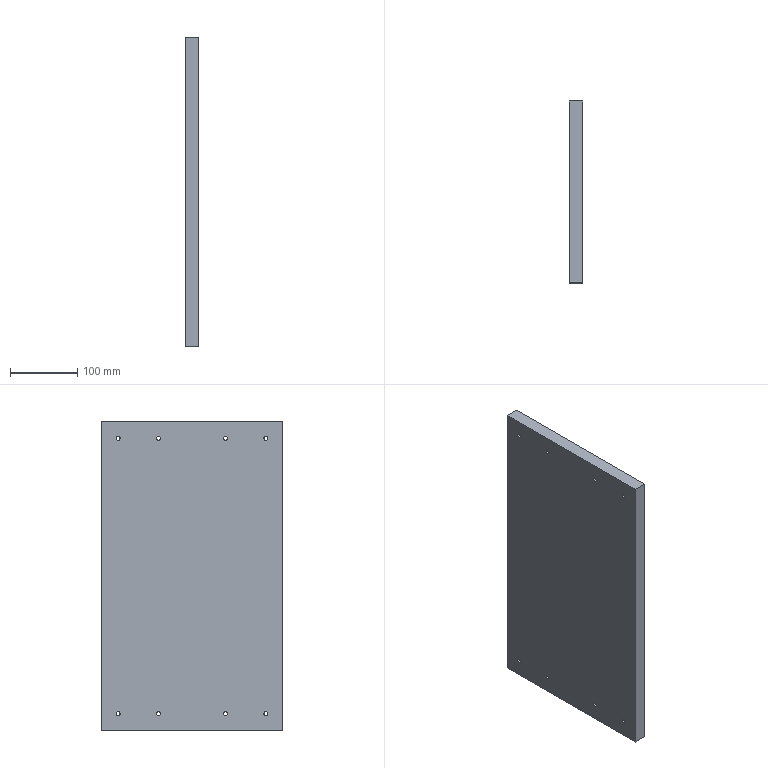Part | STEP file | Cut-Extrude 1 | 1 solid | 22 faces | box 20 x 270 x 460 mm | volume 2479476 mm3 | cylinder 16 | plane 6 | commonest cylinder face diameters 6 x16
STEP:
#1=CARTESIAN_POINT('',(-1338.738,1924.264,3010.5));
#2=VERTEX_POINT('',#1);
#3=CARTESIAN_POINT('',(-1338.738,1924.264,3016.5));
#4=VERTEX_POINT('',#3);
#5=CARTESIAN_POINT('',(-1338.738,1924.264,3013.5));
#6=DIRECTION('',(-1.,0.,0.));
#7=DIRECTION('',(0.,0.,1.));
#8=AXIS2_PLACEMENT_3D('',#5,#6,#7);
#9=CIRCLE('',#8,3.);
#10=EDGE_CURVE('',#2,#4,#9,.T.);
#11=ORIENTED_EDGE('',*,*,#10,.F.);
#12=CARTESIAN_POINT('',(-1358.738,1924.264,3010.5));
#13=VERTEX_POINT('',#12);
#14=CARTESIAN_POINT('',(-1269.738,1924.264,3010.5));
#15=DIRECTION('',(-1.,0.,0.));
#16=VECTOR('',#15,1000.);
#17=LINE('',#14,#16);
#18=EDGE_CURVE('',#2,#13,#17,.T.);
#19=ORIENTED_EDGE('',*,*,#18,.T.);
#20=CARTESIAN_POINT('',(-1358.738,1924.264,3016.5));
#21=VERTEX_POINT('',#20);
#22=CARTESIAN_POINT('',(-1358.738,1924.264,3013.5));
#23=DIRECTION('',(-1.,0.,0.));
#24=DIRECTION('',(0.,0.,-1.));
#25=AXIS2_PLACEMENT_3D('',#22,#23,#24);
#26=CIRCLE('',#25,3.);
#27=EDGE_CURVE('',#13,#21,#26,.T.);
#28=ORIENTED_EDGE('',*,*,#27,.T.);
#29=CARTESIAN_POINT('',(-1269.738,1924.264,3016.5));
#30=DIRECTION('',(-1.,0.,0.));
#31=VECTOR('',#30,1000.);
#32=LINE('',#29,#31);
#33=EDGE_CURVE('',#4,#21,#32,.T.);
#34=ORIENTED_EDGE('',*,*,#33,.F.);
#35=EDGE_LOOP('',(#11,#19,#28,#34));
#36=FACE_OUTER_BOUND('',#35,.T.);
#37=CARTESIAN_POINT('',(-1269.738,1924.264,3013.5));
#38=DIRECTION('',(-1.,0.,0.));
#39=DIRECTION('',(0.,0.,-1.));
#40=AXIS2_PLACEMENT_3D('',#37,#38,#39);
#41=CYLINDRICAL_SURFACE('',#40,3.);
#42=ADVANCED_FACE('',(#36),#41,.F.);
#43=CARTESIAN_POINT('',(-1338.738,1864.264,3010.5));
#44=VERTEX_POINT('',#43);
#45=CARTESIAN_POINT('',(-1338.738,1864.264,3016.5));
#46=VERTEX_POINT('',#45);
#47=CARTESIAN_POINT('',(-1338.738,1864.264,3013.5));
#48=DIRECTION('',(-1.,0.,0.));
#49=DIRECTION('',(0.,0.,1.));
#50=AXIS2_PLACEMENT_3D('',#47,#48,#49);
#51=CIRCLE('',#50,3.);
#52=EDGE_CURVE('',#44,#46,#51,.T.);
#53=ORIENTED_EDGE('',*,*,#52,.F.);
#54=CARTESIAN_POINT('',(-1358.738,1864.264,3010.5));
#55=VERTEX_POINT('',#54);
#56=CARTESIAN_POINT('',(-1269.738,1864.264,3010.5));
#57=DIRECTION('',(-1.,0.,0.));
#58=VECTOR('',#57,1000.);
#59=LINE('',#56,#58);
#60=EDGE_CURVE('',#44,#55,#59,.T.);
#61=ORIENTED_EDGE('',*,*,#60,.T.);
#62=CARTESIAN_POINT('',(-1358.738,1864.264,3016.5));
#63=VERTEX_POINT('',#62);
#64=CARTESIAN_POINT('',(-1358.738,1864.264,3013.5));
#65=DIRECTION('',(-1.,0.,0.));
#66=DIRECTION('',(0.,0.,-1.));
#67=AXIS2_PLACEMENT_3D('',#64,#65,#66);
#68=CIRCLE('',#67,3.);
#69=EDGE_CURVE('',#55,#63,#68,.T.);
#70=ORIENTED_EDGE('',*,*,#69,.T.);
#71=CARTESIAN_POINT('',(-1269.738,1864.264,3016.5));
#72=DIRECTION('',(-1.,0.,0.));
#73=VECTOR('',#72,1000.);
#74=LINE('',#71,#73);
#75=EDGE_CURVE('',#46,#63,#74,.T.);
#76=ORIENTED_EDGE('',*,*,#75,.F.);
#77=EDGE_LOOP('',(#53,#61,#70,#76));
#78=FACE_OUTER_BOUND('',#77,.T.);
#79=CARTESIAN_POINT('',(-1269.738,1864.264,3013.5));
#80=DIRECTION('',(-1.,0.,0.));
#81=DIRECTION('',(0.,0.,-1.));
#82=AXIS2_PLACEMENT_3D('',#79,#80,#81);
#83=CYLINDRICAL_SURFACE('',#82,3.);
#84=ADVANCED_FACE('',(#78),#83,.F.);
#85=CARTESIAN_POINT('',(-1338.738,1764.264,3010.5));
#86=VERTEX_POINT('',#85);
#87=CARTESIAN_POINT('',(-1338.738,1764.264,3016.5));
#88=VERTEX_POINT('',#87);
#89=CARTESIAN_POINT('',(-1338.738,1764.264,3013.5));
#90=DIRECTION('',(-1.,0.,0.));
#91=DIRECTION('',(0.,0.,1.));
#92=AXIS2_PLACEMENT_3D('',#89,#90,#91);
#93=CIRCLE('',#92,3.);
#94=EDGE_CURVE('',#86,#88,#93,.T.);
#95=ORIENTED_EDGE('',*,*,#94,.F.);
#96=CARTESIAN_POINT('',(-1358.738,1764.264,3010.5));
#97=VERTEX_POINT('',#96);
#98=CARTESIAN_POINT('',(-1269.738,1764.264,3010.5));
#99=DIRECTION('',(-1.,0.,0.));
#100=VECTOR('',#99,1000.);
#101=LINE('',#98,#100);
#102=EDGE_CURVE('',#86,#97,#101,.T.);
#103=ORIENTED_EDGE('',*,*,#102,.T.);
#104=CARTESIAN_POINT('',(-1358.738,1764.264,3016.5));
#105=VERTEX_POINT('',#104);
#106=CARTESIAN_POINT('',(-1358.738,1764.264,3013.5));
#107=DIRECTION('',(-1.,0.,0.));
#108=DIRECTION('',(0.,0.,1.));
#109=AXIS2_PLACEMENT_3D('',#106,#107,#108);
#110=CIRCLE('',#109,3.);
#111=EDGE_CURVE('',#97,#105,#110,.T.);
#112=ORIENTED_EDGE('',*,*,#111,.T.);
#113=CARTESIAN_POINT('',(-1269.738,1764.264,3016.5));
#114=DIRECTION('',(-1.,0.,0.));
#115=VECTOR('',#114,1000.);
#116=LINE('',#113,#115);
#117=EDGE_CURVE('',#88,#105,#116,.T.);
#118=ORIENTED_EDGE('',*,*,#117,.F.);
#119=EDGE_LOOP('',(#95,#103,#112,#118));
#120=FACE_OUTER_BOUND('',#119,.T.);
#121=CARTESIAN_POINT('',(-1269.738,1764.264,3013.5));
#122=DIRECTION('',(-1.,0.,0.));
#123=DIRECTION('',(0.,0.,-1.));
#124=AXIS2_PLACEMENT_3D('',#121,#122,#123);
#125=CYLINDRICAL_SURFACE('',#124,3.);
#126=ADVANCED_FACE('',(#120),#125,.F.);
#127=CARTESIAN_POINT('',(-1338.738,1704.264,3010.5));
#128=VERTEX_POINT('',#127);
#129=CARTESIAN_POINT('',(-1338.738,1704.264,3016.5));
#130=VERTEX_POINT('',#129);
#131=CARTESIAN_POINT('',(-1338.738,1704.264,3013.5));
#132=DIRECTION('',(-1.,0.,0.));
#133=DIRECTION('',(0.,0.,1.));
#134=AXIS2_PLACEMENT_3D('',#131,#132,#133);
#135=CIRCLE('',#134,3.);
#136=EDGE_CURVE('',#128,#130,#135,.T.);
#137=ORIENTED_EDGE('',*,*,#136,.F.);
#138=CARTESIAN_POINT('',(-1358.738,1704.264,3010.5));
#139=VERTEX_POINT('',#138);
#140=CARTESIAN_POINT('',(-1269.738,1704.264,3010.5));
#141=DIRECTION('',(-1.,0.,0.));
#142=VECTOR('',#141,1000.);
#143=LINE('',#140,#142);
#144=EDGE_CURVE('',#128,#139,#143,.T.);
#145=ORIENTED_EDGE('',*,*,#144,.T.);
#146=CARTESIAN_POINT('',(-1358.738,1704.264,3016.5));
#147=VERTEX_POINT('',#146);
#148=CARTESIAN_POINT('',(-1358.738,1704.264,3013.5));
#149=DIRECTION('',(-1.,0.,0.));
#150=DIRECTION('',(0.,0.,1.));
#151=AXIS2_PLACEMENT_3D('',#148,#149,#150);
#152=CIRCLE('',#151,3.);
#153=EDGE_CURVE('',#139,#147,#152,.T.);
#154=ORIENTED_EDGE('',*,*,#153,.T.);
#155=CARTESIAN_POINT('',(-1269.738,1704.264,3016.5));
#156=DIRECTION('',(-1.,0.,0.));
#157=VECTOR('',#156,1000.);
#158=LINE('',#155,#157);
#159=EDGE_CURVE('',#130,#147,#158,.T.);
#160=ORIENTED_EDGE('',*,*,#159,.F.);
#161=EDGE_LOOP('',(#137,#145,#154,#160));
#162=FACE_OUTER_BOUND('',#161,.T.);
#163=CARTESIAN_POINT('',(-1269.738,1704.264,3013.5));
#164=DIRECTION('',(-1.,0.,0.));
#165=DIRECTION('',(0.,0.,-1.));
#166=AXIS2_PLACEMENT_3D('',#163,#164,#165);
#167=CYLINDRICAL_SURFACE('',#166,3.);
#168=ADVANCED_FACE('',(#162),#167,.F.);
#169=CARTESIAN_POINT('',(-1338.738,1704.264,2600.5));
#170=VERTEX_POINT('',#169);
#171=CARTESIAN_POINT('',(-1338.738,1704.264,2606.5));
#172=VERTEX_POINT('',#171);
#173=CARTESIAN_POINT('',(-1338.738,1704.264,2603.5));
#174=DIRECTION('',(-1.,0.,0.));
#175=DIRECTION('',(0.,0.,1.));
#176=AXIS2_PLACEMENT_3D('',#173,#174,#175);
#177=CIRCLE('',#176,3.);
#178=EDGE_CURVE('',#170,#172,#177,.T.);
#179=ORIENTED_EDGE('',*,*,#178,.F.);
#180=CARTESIAN_POINT('',(-1358.738,1704.264,2600.5));
#181=VERTEX_POINT('',#180);
#182=CARTESIAN_POINT('',(-1269.738,1704.264,2600.5));
#183=DIRECTION('',(-1.,0.,0.));
#184=VECTOR('',#183,1000.);
#185=LINE('',#182,#184);
#186=EDGE_CURVE('',#170,#181,#185,.T.);
#187=ORIENTED_EDGE('',*,*,#186,.T.);
#188=CARTESIAN_POINT('',(-1358.738,1704.264,2606.5));
#189=VERTEX_POINT('',#188);
#190=CARTESIAN_POINT('',(-1358.738,1704.264,2603.5));
#191=DIRECTION('',(-1.,0.,0.));
#192=DIRECTION('',(0.,0.,-1.));
#193=AXIS2_PLACEMENT_3D('',#190,#191,#192);
#194=CIRCLE('',#193,3.);
#195=EDGE_CURVE('',#181,#189,#194,.T.);
#196=ORIENTED_EDGE('',*,*,#195,.T.);
#197=CARTESIAN_POINT('',(-1269.738,1704.264,2606.5));
#198=DIRECTION('',(-1.,0.,0.));
#199=VECTOR('',#198,1000.);
#200=LINE('',#197,#199);
#201=EDGE_CURVE('',#172,#189,#200,.T.);
#202=ORIENTED_EDGE('',*,*,#201,.F.);
#203=EDGE_LOOP('',(#179,#187,#196,#202));
#204=FACE_OUTER_BOUND('',#203,.T.);
#205=CARTESIAN_POINT('',(-1269.738,1704.264,2603.5));
#206=DIRECTION('',(-1.,0.,0.));
#207=DIRECTION('',(0.,0.,-1.));
#208=AXIS2_PLACEMENT_3D('',#205,#206,#207);
#209=CYLINDRICAL_SURFACE('',#208,3.);
#210=ADVANCED_FACE('',(#204),#209,.F.);
#211=CARTESIAN_POINT('',(-1338.738,1764.264,2600.5));
#212=VERTEX_POINT('',#211);
#213=CARTESIAN_POINT('',(-1338.738,1764.264,2606.5));
#214=VERTEX_POINT('',#213);
#215=CARTESIAN_POINT('',(-1338.738,1764.264,2603.5));
#216=DIRECTION('',(-1.,0.,0.));
#217=DIRECTION('',(0.,0.,1.));
#218=AXIS2_PLACEMENT_3D('',#215,#216,#217);
#219=CIRCLE('',#218,3.);
#220=EDGE_CURVE('',#212,#214,#219,.T.);
#221=ORIENTED_EDGE('',*,*,#220,.F.);
#222=CARTESIAN_POINT('',(-1358.738,1764.264,2600.5));
#223=VERTEX_POINT('',#222);
#224=CARTESIAN_POINT('',(-1269.738,1764.264,2600.5));
#225=DIRECTION('',(-1.,0.,0.));
#226=VECTOR('',#225,1000.);
#227=LINE('',#224,#226);
#228=EDGE_CURVE('',#212,#223,#227,.T.);
#229=ORIENTED_EDGE('',*,*,#228,.T.);
#230=CARTESIAN_POINT('',(-1358.738,1764.264,2606.5));
#231=VERTEX_POINT('',#230);
#232=CARTESIAN_POINT('',(-1358.738,1764.264,2603.5));
#233=DIRECTION('',(-1.,0.,0.));
#234=DIRECTION('',(0.,0.,-1.));
#235=AXIS2_PLACEMENT_3D('',#232,#233,#234);
#236=CIRCLE('',#235,3.);
#237=EDGE_CURVE('',#223,#231,#236,.T.);
#238=ORIENTED_EDGE('',*,*,#237,.T.);
#239=CARTESIAN_POINT('',(-1269.738,1764.264,2606.5));
#240=DIRECTION('',(-1.,0.,0.));
#241=VECTOR('',#240,1000.);
#242=LINE('',#239,#241);
#243=EDGE_CURVE('',#214,#231,#242,.T.);
#244=ORIENTED_EDGE('',*,*,#243,.F.);
#245=EDGE_LOOP('',(#221,#229,#238,#244));
#246=FACE_OUTER_BOUND('',#245,.T.);
#247=CARTESIAN_POINT('',(-1269.738,1764.264,2603.5));
#248=DIRECTION('',(-1.,0.,0.));
#249=DIRECTION('',(0.,0.,-1.));
#250=AXIS2_PLACEMENT_3D('',#247,#248,#249);
#251=CYLINDRICAL_SURFACE('',#250,3.);
#252=ADVANCED_FACE('',(#246),#251,.F.);
#253=CARTESIAN_POINT('',(-1338.738,1864.264,2600.5));
#254=VERTEX_POINT('',#253);
#255=CARTESIAN_POINT('',(-1338.738,1864.264,2606.5));
#256=VERTEX_POINT('',#255);
#257=CARTESIAN_POINT('',(-1338.738,1864.264,2603.5));
#258=DIRECTION('',(-1.,0.,0.));
#259=DIRECTION('',(0.,0.,1.));
#260=AXIS2_PLACEMENT_3D('',#257,#258,#259);
#261=CIRCLE('',#260,3.);
#262=EDGE_CURVE('',#254,#256,#261,.T.);
#263=ORIENTED_EDGE('',*,*,#262,.F.);
#264=CARTESIAN_POINT('',(-1358.738,1864.264,2600.5));
#265=VERTEX_POINT('',#264);
#266=CARTESIAN_POINT('',(-1269.738,1864.264,2600.5));
#267=DIRECTION('',(-1.,0.,0.));
#268=VECTOR('',#267,1000.);
#269=LINE('',#266,#268);
#270=EDGE_CURVE('',#254,#265,#269,.T.);
#271=ORIENTED_EDGE('',*,*,#270,.T.);
#272=CARTESIAN_POINT('',(-1358.738,1864.264,2606.5));
#273=VERTEX_POINT('',#272);
#274=CARTESIAN_POINT('',(-1358.738,1864.264,2603.5));
#275=DIRECTION('',(-1.,0.,0.));
#276=DIRECTION('',(0.,0.,1.));
#277=AXIS2_PLACEMENT_3D('',#274,#275,#276);
#278=CIRCLE('',#277,3.);
#279=EDGE_CURVE('',#265,#273,#278,.T.);
#280=ORIENTED_EDGE('',*,*,#279,.T.);
#281=CARTESIAN_POINT('',(-1269.738,1864.264,2606.5));
#282=DIRECTION('',(-1.,0.,0.));
#283=VECTOR('',#282,1000.);
#284=LINE('',#281,#283);
#285=EDGE_CURVE('',#256,#273,#284,.T.);
#286=ORIENTED_EDGE('',*,*,#285,.F.);
#287=EDGE_LOOP('',(#263,#271,#280,#286));
#288=FACE_OUTER_BOUND('',#287,.T.);
#289=CARTESIAN_POINT('',(-1269.738,1864.264,2603.5));
#290=DIRECTION('',(-1.,0.,0.));
#291=DIRECTION('',(0.,0.,-1.));
#292=AXIS2_PLACEMENT_3D('',#289,#290,#291);
#293=CYLINDRICAL_SURFACE('',#292,3.);
#294=ADVANCED_FACE('',(#288),#293,.F.);
#295=CARTESIAN_POINT('',(-1338.738,1924.264,2600.5));
#296=VERTEX_POINT('',#295);
#297=CARTESIAN_POINT('',(-1338.738,1924.264,2606.5));
#298=VERTEX_POINT('',#297);
#299=CARTESIAN_POINT('',(-1338.738,1924.264,2603.5));
#300=DIRECTION('',(-1.,0.,0.));
#301=DIRECTION('',(0.,0.,1.));
#302=AXIS2_PLACEMENT_3D('',#299,#300,#301);
#303=CIRCLE('',#302,3.);
#304=EDGE_CURVE('',#296,#298,#303,.T.);
#305=ORIENTED_EDGE('',*,*,#304,.F.);
#306=CARTESIAN_POINT('',(-1358.738,1924.264,2600.5));
#307=VERTEX_POINT('',#306);
#308=CARTESIAN_POINT('',(-1269.738,1924.264,2600.5));
#309=DIRECTION('',(-1.,0.,0.));
#310=VECTOR('',#309,1000.);
#311=LINE('',#308,#310);
#312=EDGE_CURVE('',#296,#307,#311,.T.);
#313=ORIENTED_EDGE('',*,*,#312,.T.);
#314=CARTESIAN_POINT('',(-1358.738,1924.264,2606.5));
#315=VERTEX_POINT('',#314);
#316=CARTESIAN_POINT('',(-1358.738,1924.264,2603.5));
#317=DIRECTION('',(-1.,0.,0.));
#318=DIRECTION('',(0.,0.,1.));
#319=AXIS2_PLACEMENT_3D('',#316,#317,#318);
#320=CIRCLE('',#319,3.);
#321=EDGE_CURVE('',#307,#315,#320,.T.);
#322=ORIENTED_EDGE('',*,*,#321,.T.);
#323=CARTESIAN_POINT('',(-1269.738,1924.264,2606.5));
#324=DIRECTION('',(-1.,0.,0.));
#325=VECTOR('',#324,1000.);
#326=LINE('',#323,#325);
#327=EDGE_CURVE('',#298,#315,#326,.T.);
#328=ORIENTED_EDGE('',*,*,#327,.F.);
#329=EDGE_LOOP('',(#305,#313,#322,#328));
#330=FACE_OUTER_BOUND('',#329,.T.);
#331=CARTESIAN_POINT('',(-1269.738,1924.264,2603.5));
#332=DIRECTION('',(-1.,0.,0.));
#333=DIRECTION('',(0.,0.,-1.));
#334=AXIS2_PLACEMENT_3D('',#331,#332,#333);
#335=CYLINDRICAL_SURFACE('',#334,3.);
#336=ADVANCED_FACE('',(#330),#335,.F.);
#337=CARTESIAN_POINT('',(-1338.738,1679.264,3038.5));
#338=VERTEX_POINT('',#337);
#339=CARTESIAN_POINT('',(-1338.738,1949.264,3038.5));
#340=VERTEX_POINT('',#339);
#341=CARTESIAN_POINT('',(-1338.738,1949.264,3038.5));
#342=DIRECTION('',(0.,1.,0.));
#343=VECTOR('',#342,1000.);
#344=LINE('',#341,#343);
#345=EDGE_CURVE('',#338,#340,#344,.T.);
#346=ORIENTED_EDGE('',*,*,#345,.T.);
#347=CARTESIAN_POINT('',(-1358.738,1949.264,3038.5));
#348=VERTEX_POINT('',#347);
#349=CARTESIAN_POINT('',(-1358.738,1949.264,3038.5));
#350=DIRECTION('',(1.,0.,0.));
#351=VECTOR('',#350,1000.);
#352=LINE('',#349,#351);
#353=EDGE_CURVE('',#348,#340,#352,.T.);
#354=ORIENTED_EDGE('',*,*,#353,.F.);
#355=CARTESIAN_POINT('',(-1358.738,1679.264,3038.5));
#356=VERTEX_POINT('',#355);
#357=CARTESIAN_POINT('',(-1358.738,1949.264,3038.5));
#358=DIRECTION('',(0.,1.,0.));
#359=VECTOR('',#358,1000.);
#360=LINE('',#357,#359);
#361=EDGE_CURVE('',#356,#348,#360,.T.);
#362=ORIENTED_EDGE('',*,*,#361,.F.);
#363=CARTESIAN_POINT('',(-1358.738,1679.264,3038.5));
#364=DIRECTION('',(1.,0.,0.));
#365=VECTOR('',#364,1000.);
#366=LINE('',#363,#365);
#367=EDGE_CURVE('',#356,#338,#366,.T.);
#368=ORIENTED_EDGE('',*,*,#367,.T.);
#369=EDGE_LOOP('',(#346,#354,#362,#368));
#370=FACE_OUTER_BOUND('',#369,.T.);
#371=CARTESIAN_POINT('',(-1358.738,1949.264,3038.5));
#372=DIRECTION('',(0.,0.,-1.));
#373=DIRECTION('',(0.,1.,0.));
#374=AXIS2_PLACEMENT_3D('',#371,#372,#373);
#375=PLANE('',#374);
#376=ADVANCED_FACE('',(#370),#375,.F.);
#377=CARTESIAN_POINT('',(-1338.738,1949.264,2578.5));
#378=VERTEX_POINT('',#377);
#379=CARTESIAN_POINT('',(-1338.738,1949.264,2578.5));
#380=DIRECTION('',(0.,0.,-1.));
#381=VECTOR('',#380,1000.);
#382=LINE('',#379,#381);
#383=EDGE_CURVE('',#340,#378,#382,.T.);
#384=ORIENTED_EDGE('',*,*,#383,.T.);
#385=CARTESIAN_POINT('',(-1358.738,1949.264,2578.5));
#386=VERTEX_POINT('',#385);
#387=CARTESIAN_POINT('',(-1358.738,1949.264,2578.5));
#388=DIRECTION('',(1.,0.,0.));
#389=VECTOR('',#388,1000.);
#390=LINE('',#387,#389);
#391=EDGE_CURVE('',#386,#378,#390,.T.);
#392=ORIENTED_EDGE('',*,*,#391,.F.);
#393=CARTESIAN_POINT('',(-1358.738,1949.264,2578.5));
#394=DIRECTION('',(0.,0.,-1.));
#395=VECTOR('',#394,1000.);
#396=LINE('',#393,#395);
#397=EDGE_CURVE('',#348,#386,#396,.T.);
#398=ORIENTED_EDGE('',*,*,#397,.F.);
#399=ORIENTED_EDGE('',*,*,#353,.T.);
#400=EDGE_LOOP('',(#384,#392,#398,#399));
#401=FACE_OUTER_BOUND('',#400,.T.);
#402=CARTESIAN_POINT('',(-1358.738,1949.264,2578.5));
#403=DIRECTION('',(0.,-1.,0.));
#404=DIRECTION('',(-1.,0.,0.));
#405=AXIS2_PLACEMENT_3D('',#402,#403,#404);
#406=PLANE('',#405);
#407=ADVANCED_FACE('',(#401),#406,.F.);
#408=CARTESIAN_POINT('',(-1338.738,1679.264,2578.5));
#409=VERTEX_POINT('',#408);
#410=CARTESIAN_POINT('',(-1338.738,1949.264,2578.5));
#411=DIRECTION('',(0.,-1.,0.));
#412=VECTOR('',#411,1000.);
#413=LINE('',#410,#412);
#414=EDGE_CURVE('',#378,#409,#413,.T.);
#415=ORIENTED_EDGE('',*,*,#414,.T.);
#416=CARTESIAN_POINT('',(-1358.738,1679.264,2578.5));
#417=VERTEX_POINT('',#416);
#418=CARTESIAN_POINT('',(-1358.738,1679.264,2578.5));
#419=DIRECTION('',(1.,0.,0.));
#420=VECTOR('',#419,1000.);
#421=LINE('',#418,#420);
#422=EDGE_CURVE('',#417,#409,#421,.T.);
#423=ORIENTED_EDGE('',*,*,#422,.F.);
#424=CARTESIAN_POINT('',(-1358.738,1949.264,2578.5));
#425=DIRECTION('',(0.,-1.,0.));
#426=VECTOR('',#425,1000.);
#427=LINE('',#424,#426);
#428=EDGE_CURVE('',#386,#417,#427,.T.);
#429=ORIENTED_EDGE('',*,*,#428,.F.);
#430=ORIENTED_EDGE('',*,*,#391,.T.);
#431=EDGE_LOOP('',(#415,#423,#429,#430));
#432=FACE_OUTER_BOUND('',#431,.T.);
#433=CARTESIAN_POINT('',(-1358.738,1949.264,2578.5));
#434=DIRECTION('',(0.,0.,1.));
#435=DIRECTION('',(0.,-1.,0.));
#436=AXIS2_PLACEMENT_3D('',#433,#434,#435);
#437=PLANE('',#436);
#438=ADVANCED_FACE('',(#432),#437,.F.);
#439=CARTESIAN_POINT('',(-1338.738,1679.264,2578.5));
#440=DIRECTION('',(0.,0.,1.));
#441=VECTOR('',#440,1000.);
#442=LINE('',#439,#441);
#443=EDGE_CURVE('',#409,#338,#442,.T.);
#444=ORIENTED_EDGE('',*,*,#443,.T.);
#445=ORIENTED_EDGE('',*,*,#367,.F.);
#446=CARTESIAN_POINT('',(-1358.738,1679.264,2578.5));
#447=DIRECTION('',(0.,0.,1.));
#448=VECTOR('',#447,1000.);
#449=LINE('',#446,#448);
#450=EDGE_CURVE('',#417,#356,#449,.T.);
#451=ORIENTED_EDGE('',*,*,#450,.F.);
#452=ORIENTED_EDGE('',*,*,#422,.T.);
#453=EDGE_LOOP('',(#444,#445,#451,#452));
#454=FACE_OUTER_BOUND('',#453,.T.);
#455=CARTESIAN_POINT('',(-1358.738,1679.264,2578.5));
#456=DIRECTION('',(0.,1.,0.));
#457=DIRECTION('',(1.,0.,0.));
#458=AXIS2_PLACEMENT_3D('',#455,#456,#457);
#459=PLANE('',#458);
#460=ADVANCED_FACE('',(#454),#459,.F.);
#461=CARTESIAN_POINT('',(-1358.738,1924.264,3013.5));
#462=DIRECTION('',(-1.,0.,0.));
#463=DIRECTION('',(0.,0.,-1.));
#464=AXIS2_PLACEMENT_3D('',#461,#462,#463);
#465=CIRCLE('',#464,3.);
#466=EDGE_CURVE('',#21,#13,#465,.T.);
#467=ORIENTED_EDGE('',*,*,#466,.F.);
#468=ORIENTED_EDGE('',*,*,#27,.F.);
#469=EDGE_LOOP('',(#467,#468));
#470=FACE_BOUND('',#469,.T.);
#471=CARTESIAN_POINT('',(-1358.738,1864.264,3013.5));
#472=DIRECTION('',(-1.,0.,0.));
#473=DIRECTION('',(0.,0.,-1.));
#474=AXIS2_PLACEMENT_3D('',#471,#472,#473);
#475=CIRCLE('',#474,3.);
#476=EDGE_CURVE('',#63,#55,#475,.T.);
#477=ORIENTED_EDGE('',*,*,#476,.F.);
#478=ORIENTED_EDGE('',*,*,#69,.F.);
#479=EDGE_LOOP('',(#477,#478));
#480=FACE_BOUND('',#479,.T.);
#481=CARTESIAN_POINT('',(-1358.738,1764.264,3013.5));
#482=DIRECTION('',(-1.,0.,0.));
#483=DIRECTION('',(0.,0.,1.));
#484=AXIS2_PLACEMENT_3D('',#481,#482,#483);
#485=CIRCLE('',#484,3.);
#486=EDGE_CURVE('',#105,#97,#485,.T.);
#487=ORIENTED_EDGE('',*,*,#486,.F.);
#488=ORIENTED_EDGE('',*,*,#111,.F.);
#489=EDGE_LOOP('',(#487,#488));
#490=FACE_BOUND('',#489,.T.);
#491=CARTESIAN_POINT('',(-1358.738,1704.264,3013.5));
#492=DIRECTION('',(-1.,0.,0.));
#493=DIRECTION('',(0.,0.,1.));
#494=AXIS2_PLACEMENT_3D('',#491,#492,#493);
#495=CIRCLE('',#494,3.);
#496=EDGE_CURVE('',#147,#139,#495,.T.);
#497=ORIENTED_EDGE('',*,*,#496,.F.);
#498=ORIENTED_EDGE('',*,*,#153,.F.);
#499=EDGE_LOOP('',(#497,#498));
#500=FACE_BOUND('',#499,.T.);
#501=CARTESIAN_POINT('',(-1358.738,1704.264,2603.5));
#502=DIRECTION('',(-1.,0.,0.));
#503=DIRECTION('',(0.,0.,-1.));
#504=AXIS2_PLACEMENT_3D('',#501,#502,#503);
#505=CIRCLE('',#504,3.);
#506=EDGE_CURVE('',#189,#181,#505,.T.);
#507=ORIENTED_EDGE('',*,*,#506,.F.);
#508=ORIENTED_EDGE('',*,*,#195,.F.);
#509=EDGE_LOOP('',(#507,#508));
#510=FACE_BOUND('',#509,.T.);
#511=CARTESIAN_POINT('',(-1358.738,1764.264,2603.5));
#512=DIRECTION('',(-1.,0.,0.));
#513=DIRECTION('',(0.,0.,-1.));
#514=AXIS2_PLACEMENT_3D('',#511,#512,#513);
#515=CIRCLE('',#514,3.);
#516=EDGE_CURVE('',#231,#223,#515,.T.);
#517=ORIENTED_EDGE('',*,*,#516,.F.);
#518=ORIENTED_EDGE('',*,*,#237,.F.);
#519=EDGE_LOOP('',(#517,#518));
#520=FACE_BOUND('',#519,.T.);
#521=CARTESIAN_POINT('',(-1358.738,1864.264,2603.5));
#522=DIRECTION('',(-1.,0.,0.));
#523=DIRECTION('',(0.,0.,1.));
#524=AXIS2_PLACEMENT_3D('',#521,#522,#523);
#525=CIRCLE('',#524,3.);
#526=EDGE_CURVE('',#273,#265,#525,.T.);
#527=ORIENTED_EDGE('',*,*,#526,.F.);
#528=ORIENTED_EDGE('',*,*,#279,.F.);
#529=EDGE_LOOP('',(#527,#528));
#530=FACE_BOUND('',#529,.T.);
#531=CARTESIAN_POINT('',(-1358.738,1924.264,2603.5));
#532=DIRECTION('',(-1.,0.,0.));
#533=DIRECTION('',(0.,0.,1.));
#534=AXIS2_PLACEMENT_3D('',#531,#532,#533);
#535=CIRCLE('',#534,3.);
#536=EDGE_CURVE('',#315,#307,#535,.T.);
#537=ORIENTED_EDGE('',*,*,#536,.F.);
#538=ORIENTED_EDGE('',*,*,#321,.F.);
#539=EDGE_LOOP('',(#537,#538));
#540=FACE_BOUND('',#539,.T.);
#541=ORIENTED_EDGE('',*,*,#361,.T.);
#542=ORIENTED_EDGE('',*,*,#397,.T.);
#543=ORIENTED_EDGE('',*,*,#428,.T.);
#544=ORIENTED_EDGE('',*,*,#450,.T.);
#545=EDGE_LOOP('',(#541,#542,#543,#544));
#546=FACE_OUTER_BOUND('',#545,.T.);
#547=CARTESIAN_POINT('',(-1358.738,1814.264,2808.5));
#548=DIRECTION('',(-1.,0.,0.));
#549=DIRECTION('',(0.,0.,-1.));
#550=AXIS2_PLACEMENT_3D('',#547,#548,#549);
#551=PLANE('',#550);
#552=ADVANCED_FACE('',(#470,#480,#490,#500,#510,#520,#530,#540,#546),#551,.T.);
#553=CARTESIAN_POINT('',(-1338.738,1924.264,3013.5));
#554=DIRECTION('',(-1.,0.,0.));
#555=DIRECTION('',(0.,0.,1.));
#556=AXIS2_PLACEMENT_3D('',#553,#554,#555);
#557=CIRCLE('',#556,3.);
#558=EDGE_CURVE('',#4,#2,#557,.T.);
#559=ORIENTED_EDGE('',*,*,#558,.T.);
#560=ORIENTED_EDGE('',*,*,#10,.T.);
#561=EDGE_LOOP('',(#559,#560));
#562=FACE_BOUND('',#561,.T.);
#563=CARTESIAN_POINT('',(-1338.738,1864.264,3013.5));
#564=DIRECTION('',(-1.,0.,0.));
#565=DIRECTION('',(0.,0.,1.));
#566=AXIS2_PLACEMENT_3D('',#563,#564,#565);
#567=CIRCLE('',#566,3.);
#568=EDGE_CURVE('',#46,#44,#567,.T.);
#569=ORIENTED_EDGE('',*,*,#568,.T.);
#570=ORIENTED_EDGE('',*,*,#52,.T.);
#571=EDGE_LOOP('',(#569,#570));
#572=FACE_BOUND('',#571,.T.);
#573=CARTESIAN_POINT('',(-1338.738,1764.264,3013.5));
#574=DIRECTION('',(-1.,0.,0.));
#575=DIRECTION('',(0.,0.,1.));
#576=AXIS2_PLACEMENT_3D('',#573,#574,#575);
#577=CIRCLE('',#576,3.);
#578=EDGE_CURVE('',#88,#86,#577,.T.);
#579=ORIENTED_EDGE('',*,*,#578,.T.);
#580=ORIENTED_EDGE('',*,*,#94,.T.);
#581=EDGE_LOOP('',(#579,#580));
#582=FACE_BOUND('',#581,.T.);
#583=CARTESIAN_POINT('',(-1338.738,1704.264,3013.5));
#584=DIRECTION('',(-1.,0.,0.));
#585=DIRECTION('',(0.,0.,1.));
#586=AXIS2_PLACEMENT_3D('',#583,#584,#585);
#587=CIRCLE('',#586,3.);
#588=EDGE_CURVE('',#130,#128,#587,.T.);
#589=ORIENTED_EDGE('',*,*,#588,.T.);
#590=ORIENTED_EDGE('',*,*,#136,.T.);
#591=EDGE_LOOP('',(#589,#590));
#592=FACE_BOUND('',#591,.T.);
#593=CARTESIAN_POINT('',(-1338.738,1704.264,2603.5));
#594=DIRECTION('',(-1.,0.,0.));
#595=DIRECTION('',(0.,0.,1.));
#596=AXIS2_PLACEMENT_3D('',#593,#594,#595);
#597=CIRCLE('',#596,3.);
#598=EDGE_CURVE('',#172,#170,#597,.T.);
#599=ORIENTED_EDGE('',*,*,#598,.T.);
#600=ORIENTED_EDGE('',*,*,#178,.T.);
#601=EDGE_LOOP('',(#599,#600));
#602=FACE_BOUND('',#601,.T.);
#603=CARTESIAN_POINT('',(-1338.738,1764.264,2603.5));
#604=DIRECTION('',(-1.,0.,0.));
#605=DIRECTION('',(0.,0.,1.));
#606=AXIS2_PLACEMENT_3D('',#603,#604,#605);
#607=CIRCLE('',#606,3.);
#608=EDGE_CURVE('',#214,#212,#607,.T.);
#609=ORIENTED_EDGE('',*,*,#608,.T.);
#610=ORIENTED_EDGE('',*,*,#220,.T.);
#611=EDGE_LOOP('',(#609,#610));
#612=FACE_BOUND('',#611,.T.);
#613=CARTESIAN_POINT('',(-1338.738,1864.264,2603.5));
#614=DIRECTION('',(-1.,0.,0.));
#615=DIRECTION('',(0.,0.,1.));
#616=AXIS2_PLACEMENT_3D('',#613,#614,#615);
#617=CIRCLE('',#616,3.);
#618=EDGE_CURVE('',#256,#254,#617,.T.);
#619=ORIENTED_EDGE('',*,*,#618,.T.);
#620=ORIENTED_EDGE('',*,*,#262,.T.);
#621=EDGE_LOOP('',(#619,#620));
#622=FACE_BOUND('',#621,.T.);
#623=CARTESIAN_POINT('',(-1338.738,1924.264,2603.5));
#624=DIRECTION('',(-1.,0.,0.));
#625=DIRECTION('',(0.,0.,1.));
#626=AXIS2_PLACEMENT_3D('',#623,#624,#625);
#627=CIRCLE('',#626,3.);
#628=EDGE_CURVE('',#298,#296,#627,.T.);
#629=ORIENTED_EDGE('',*,*,#628,.T.);
#630=ORIENTED_EDGE('',*,*,#304,.T.);
#631=EDGE_LOOP('',(#629,#630));
#632=FACE_BOUND('',#631,.T.);
#633=ORIENTED_EDGE('',*,*,#345,.F.);
#634=ORIENTED_EDGE('',*,*,#443,.F.);
#635=ORIENTED_EDGE('',*,*,#414,.F.);
#636=ORIENTED_EDGE('',*,*,#383,.F.);
#637=EDGE_LOOP('',(#633,#634,#635,#636));
#638=FACE_OUTER_BOUND('',#637,.T.);
#639=CARTESIAN_POINT('',(-1338.738,1814.264,2808.5));
#640=DIRECTION('',(-1.,0.,0.));
#641=DIRECTION('',(0.,0.,-1.));
#642=AXIS2_PLACEMENT_3D('',#639,#640,#641);
#643=PLANE('',#642);
#644=ADVANCED_FACE('',(#562,#572,#582,#592,#602,#612,#622,#632,#638),#643,.F.);
#645=ORIENTED_EDGE('',*,*,#312,.F.);
#646=ORIENTED_EDGE('',*,*,#628,.F.);
#647=ORIENTED_EDGE('',*,*,#327,.T.);
#648=ORIENTED_EDGE('',*,*,#536,.T.);
#649=EDGE_LOOP('',(#645,#646,#647,#648));
#650=FACE_OUTER_BOUND('',#649,.T.);
#651=CARTESIAN_POINT('',(-1269.738,1924.264,2603.5));
#652=DIRECTION('',(-1.,0.,0.));
#653=DIRECTION('',(0.,0.,-1.));
#654=AXIS2_PLACEMENT_3D('',#651,#652,#653);
#655=CYLINDRICAL_SURFACE('',#654,3.);
#656=ADVANCED_FACE('',(#650),#655,.F.);
#657=ORIENTED_EDGE('',*,*,#270,.F.);
#658=ORIENTED_EDGE('',*,*,#618,.F.);
#659=ORIENTED_EDGE('',*,*,#285,.T.);
#660=ORIENTED_EDGE('',*,*,#526,.T.);
#661=EDGE_LOOP('',(#657,#658,#659,#660));
#662=FACE_OUTER_BOUND('',#661,.T.);
#663=CARTESIAN_POINT('',(-1269.738,1864.264,2603.5));
#664=DIRECTION('',(-1.,0.,0.));
#665=DIRECTION('',(0.,0.,-1.));
#666=AXIS2_PLACEMENT_3D('',#663,#664,#665);
#667=CYLINDRICAL_SURFACE('',#666,3.);
#668=ADVANCED_FACE('',(#662),#667,.F.);
#669=ORIENTED_EDGE('',*,*,#228,.F.);
#670=ORIENTED_EDGE('',*,*,#608,.F.);
#671=ORIENTED_EDGE('',*,*,#243,.T.);
#672=ORIENTED_EDGE('',*,*,#516,.T.);
#673=EDGE_LOOP('',(#669,#670,#671,#672));
#674=FACE_OUTER_BOUND('',#673,.T.);
#675=CARTESIAN_POINT('',(-1269.738,1764.264,2603.5));
#676=DIRECTION('',(-1.,0.,0.));
#677=DIRECTION('',(0.,0.,-1.));
#678=AXIS2_PLACEMENT_3D('',#675,#676,#677);
#679=CYLINDRICAL_SURFACE('',#678,3.);
#680=ADVANCED_FACE('',(#674),#679,.F.);
#681=ORIENTED_EDGE('',*,*,#186,.F.);
#682=ORIENTED_EDGE('',*,*,#598,.F.);
#683=ORIENTED_EDGE('',*,*,#201,.T.);
#684=ORIENTED_EDGE('',*,*,#506,.T.);
#685=EDGE_LOOP('',(#681,#682,#683,#684));
#686=FACE_OUTER_BOUND('',#685,.T.);
#687=CARTESIAN_POINT('',(-1269.738,1704.264,2603.5));
#688=DIRECTION('',(-1.,0.,0.));
#689=DIRECTION('',(0.,0.,-1.));
#690=AXIS2_PLACEMENT_3D('',#687,#688,#689);
#691=CYLINDRICAL_SURFACE('',#690,3.);
#692=ADVANCED_FACE('',(#686),#691,.F.);
#693=ORIENTED_EDGE('',*,*,#144,.F.);
#694=ORIENTED_EDGE('',*,*,#588,.F.);
#695=ORIENTED_EDGE('',*,*,#159,.T.);
#696=ORIENTED_EDGE('',*,*,#496,.T.);
#697=EDGE_LOOP('',(#693,#694,#695,#696));
#698=FACE_OUTER_BOUND('',#697,.T.);
#699=CARTESIAN_POINT('',(-1269.738,1704.264,3013.5));
#700=DIRECTION('',(-1.,0.,0.));
#701=DIRECTION('',(0.,0.,-1.));
#702=AXIS2_PLACEMENT_3D('',#699,#700,#701);
#703=CYLINDRICAL_SURFACE('',#702,3.);
#704=ADVANCED_FACE('',(#698),#703,.F.);
#705=ORIENTED_EDGE('',*,*,#102,.F.);
#706=ORIENTED_EDGE('',*,*,#578,.F.);
#707=ORIENTED_EDGE('',*,*,#117,.T.);
#708=ORIENTED_EDGE('',*,*,#486,.T.);
#709=EDGE_LOOP('',(#705,#706,#707,#708));
#710=FACE_OUTER_BOUND('',#709,.T.);
#711=CARTESIAN_POINT('',(-1269.738,1764.264,3013.5));
#712=DIRECTION('',(-1.,0.,0.));
#713=DIRECTION('',(0.,0.,-1.));
#714=AXIS2_PLACEMENT_3D('',#711,#712,#713);
#715=CYLINDRICAL_SURFACE('',#714,3.);
#716=ADVANCED_FACE('',(#710),#715,.F.);
#717=ORIENTED_EDGE('',*,*,#60,.F.);
#718=ORIENTED_EDGE('',*,*,#568,.F.);
#719=ORIENTED_EDGE('',*,*,#75,.T.);
#720=ORIENTED_EDGE('',*,*,#476,.T.);
#721=EDGE_LOOP('',(#717,#718,#719,#720));
#722=FACE_OUTER_BOUND('',#721,.T.);
#723=CARTESIAN_POINT('',(-1269.738,1864.264,3013.5));
#724=DIRECTION('',(-1.,0.,0.));
#725=DIRECTION('',(0.,0.,-1.));
#726=AXIS2_PLACEMENT_3D('',#723,#724,#725);
#727=CYLINDRICAL_SURFACE('',#726,3.);
#728=ADVANCED_FACE('',(#722),#727,.F.);
#729=ORIENTED_EDGE('',*,*,#18,.F.);
#730=ORIENTED_EDGE('',*,*,#558,.F.);
#731=ORIENTED_EDGE('',*,*,#33,.T.);
#732=ORIENTED_EDGE('',*,*,#466,.T.);
#733=EDGE_LOOP('',(#729,#730,#731,#732));
#734=FACE_OUTER_BOUND('',#733,.T.);
#735=CARTESIAN_POINT('',(-1269.738,1924.264,3013.5));
#736=DIRECTION('',(-1.,0.,0.));
#737=DIRECTION('',(0.,0.,-1.));
#738=AXIS2_PLACEMENT_3D('',#735,#736,#737);
#739=CYLINDRICAL_SURFACE('',#738,3.);
#740=ADVANCED_FACE('',(#734),#739,.F.);
#741=CLOSED_SHELL('',(#42,#84,#126,#168,#210,#252,#294,#336,#376,#407,#438,#460,#552,#644,#656,#668,#680,#692,#704,#716,#728,#740));
#742=MANIFOLD_SOLID_BREP('',#741);
#743=CARTESIAN_POINT('',(0.,0.,0.));
#744=DIRECTION('',(0.,0.,1.));
#745=DIRECTION('',(1.,0.,0.));
#746=AXIS2_PLACEMENT_3D('',#743,#744,#745);
#747=(LENGTH_UNIT()NAMED_UNIT(*)SI_UNIT(.MILLI.,.METRE.));
#748=UNCERTAINTY_MEASURE_WITH_UNIT(LENGTH_MEASURE(0.00001),#747,'','');
#749=(NAMED_UNIT(*)PLANE_ANGLE_UNIT()SI_UNIT($,.RADIAN.));
#750=(NAMED_UNIT(*)SI_UNIT($,.STERADIAN.)SOLID_ANGLE_UNIT());
#751=(GEOMETRIC_REPRESENTATION_CONTEXT(3)GLOBAL_UNCERTAINTY_ASSIGNED_CONTEXT((#748))GLOBAL_UNIT_ASSIGNED_CONTEXT((#747,#749,#750))REPRESENTATION_CONTEXT('',''));
#752=ADVANCED_BREP_SHAPE_REPRESENTATION('',(#742,#746),#751);